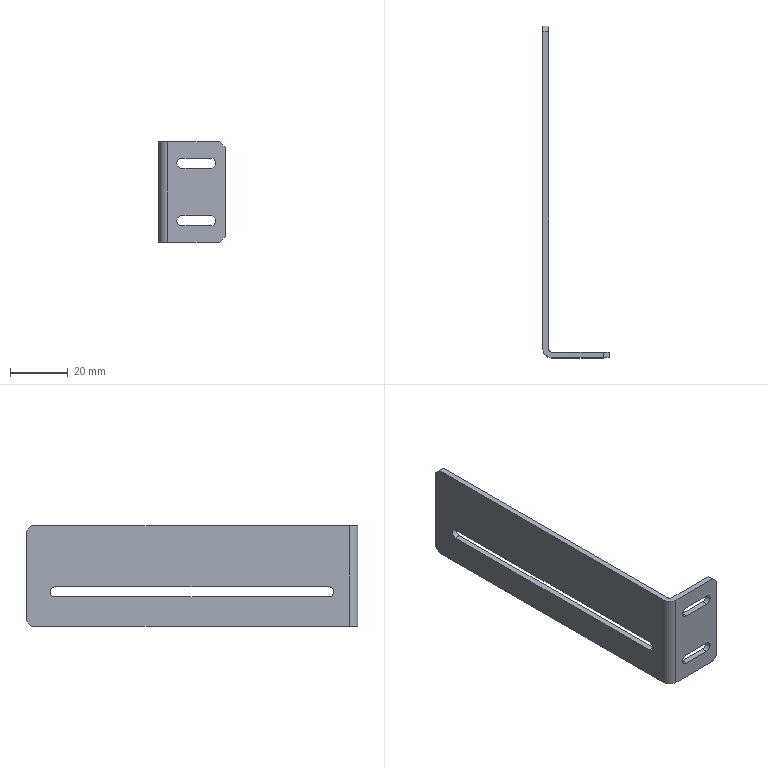Part | SolidWorks | features BaseBody 1 | 1 solid | 27 faces | box 23 x 115 x 35 mm | volume 8601 mm3 | plane 18 | cylinder 9 | commonest cylinder face diameters 3.5 x4 3.4 x3 2 x1 6 x1
STEP:
#1=CARTESIAN_POINT('',(-11.,6.3,-5.5));
#2=VERTEX_POINT('',#1);
#3=CARTESIAN_POINT('',(-11.,8.,-3.8));
#4=VERTEX_POINT('',#3);
#5=CARTESIAN_POINT('',(-11.,8.,-5.5));
#6=DIRECTION('',(-1.,0.,0.));
#7=DIRECTION('',(0.,1.,0.));
#8=AXIS2_PLACEMENT_3D('',#5,#6,#7);
#9=CIRCLE('',#8,1.7);
#10=EDGE_CURVE('',#2,#4,#9,.T.);
#11=ORIENTED_EDGE('',*,*,#10,.F.);
#12=CARTESIAN_POINT('',(-13.,6.3,-5.5));
#13=VERTEX_POINT('',#12);
#14=CARTESIAN_POINT('',(10.001,6.3,-5.5));
#15=DIRECTION('',(-1.,0.,0.));
#16=VECTOR('',#15,1000.);
#17=LINE('',#14,#16);
#18=EDGE_CURVE('',#2,#13,#17,.T.);
#19=ORIENTED_EDGE('',*,*,#18,.T.);
#20=CARTESIAN_POINT('',(-13.,8.,-3.8));
#21=VERTEX_POINT('',#20);
#22=CARTESIAN_POINT('',(-13.,8.,-5.5));
#23=DIRECTION('',(-1.,0.,0.));
#24=DIRECTION('',(0.,-1.,0.));
#25=AXIS2_PLACEMENT_3D('',#22,#23,#24);
#26=CIRCLE('',#25,1.7);
#27=EDGE_CURVE('',#13,#21,#26,.T.);
#28=ORIENTED_EDGE('',*,*,#27,.T.);
#29=CARTESIAN_POINT('',(10.001,8.,-3.8));
#30=DIRECTION('',(-1.,0.,0.));
#31=VECTOR('',#30,1000.);
#32=LINE('',#29,#31);
#33=EDGE_CURVE('',#4,#21,#32,.T.);
#34=ORIENTED_EDGE('',*,*,#33,.F.);
#35=EDGE_LOOP('',(#11,#19,#28,#34));
#36=FACE_OUTER_BOUND('',#35,.T.);
#37=CARTESIAN_POINT('',(10.001,8.,-5.5));
#38=DIRECTION('',(-1.,0.,0.));
#39=DIRECTION('',(0.,-1.,0.));
#40=AXIS2_PLACEMENT_3D('',#37,#38,#39);
#41=CYLINDRICAL_SURFACE('',#40,1.7);
#42=ADVANCED_FACE('',(#36),#41,.F.);
#43=ORIENTED_EDGE('',*,*,#33,.T.);
#44=CARTESIAN_POINT('',(-13.,103.,-3.8));
#45=VERTEX_POINT('',#44);
#46=CARTESIAN_POINT('',(-13.,8.,-3.8));
#47=DIRECTION('',(0.,1.,0.));
#48=VECTOR('',#47,1000.);
#49=LINE('',#46,#48);
#50=EDGE_CURVE('',#21,#45,#49,.T.);
#51=ORIENTED_EDGE('',*,*,#50,.T.);
#52=CARTESIAN_POINT('',(-11.,103.,-3.8));
#53=VERTEX_POINT('',#52);
#54=CARTESIAN_POINT('',(10.001,103.,-3.8));
#55=DIRECTION('',(-1.,0.,0.));
#56=VECTOR('',#55,1000.);
#57=LINE('',#54,#56);
#58=EDGE_CURVE('',#53,#45,#57,.T.);
#59=ORIENTED_EDGE('',*,*,#58,.F.);
#60=CARTESIAN_POINT('',(-11.,8.,-3.8));
#61=DIRECTION('',(0.,1.,0.));
#62=VECTOR('',#61,1000.);
#63=LINE('',#60,#62);
#64=EDGE_CURVE('',#4,#53,#63,.T.);
#65=ORIENTED_EDGE('',*,*,#64,.F.);
#66=EDGE_LOOP('',(#43,#51,#59,#65));
#67=FACE_OUTER_BOUND('',#66,.T.);
#68=CARTESIAN_POINT('',(10.001,8.,-3.8));
#69=DIRECTION('',(0.,0.,1.));
#70=DIRECTION('',(1.,0.,0.));
#71=AXIS2_PLACEMENT_3D('',#68,#69,#70);
#72=PLANE('',#71);
#73=ADVANCED_FACE('',(#67),#72,.F.);
#74=ORIENTED_EDGE('',*,*,#58,.T.);
#75=CARTESIAN_POINT('',(-13.,103.,-7.2));
#76=VERTEX_POINT('',#75);
#77=CARTESIAN_POINT('',(-13.,103.,-5.5));
#78=DIRECTION('',(-1.,0.,0.));
#79=DIRECTION('',(0.,-1.,0.));
#80=AXIS2_PLACEMENT_3D('',#77,#78,#79);
#81=CIRCLE('',#80,1.7);
#82=EDGE_CURVE('',#45,#76,#81,.T.);
#83=ORIENTED_EDGE('',*,*,#82,.T.);
#84=CARTESIAN_POINT('',(-11.,103.,-7.2));
#85=VERTEX_POINT('',#84);
#86=CARTESIAN_POINT('',(10.001,103.,-7.2));
#87=DIRECTION('',(-1.,0.,0.));
#88=VECTOR('',#87,1000.);
#89=LINE('',#86,#88);
#90=EDGE_CURVE('',#85,#76,#89,.T.);
#91=ORIENTED_EDGE('',*,*,#90,.F.);
#92=CARTESIAN_POINT('',(-11.,103.,-5.5));
#93=DIRECTION('',(-1.,0.,0.));
#94=DIRECTION('',(0.,1.,0.));
#95=AXIS2_PLACEMENT_3D('',#92,#93,#94);
#96=CIRCLE('',#95,1.7);
#97=EDGE_CURVE('',#53,#85,#96,.T.);
#98=ORIENTED_EDGE('',*,*,#97,.F.);
#99=EDGE_LOOP('',(#74,#83,#91,#98));
#100=FACE_OUTER_BOUND('',#99,.T.);
#101=CARTESIAN_POINT('',(10.001,103.,-5.5));
#102=DIRECTION('',(-1.,0.,0.));
#103=DIRECTION('',(0.,-1.,0.));
#104=AXIS2_PLACEMENT_3D('',#101,#102,#103);
#105=CYLINDRICAL_SURFACE('',#104,1.7);
#106=ADVANCED_FACE('',(#100),#105,.F.);
#107=ORIENTED_EDGE('',*,*,#90,.T.);
#108=CARTESIAN_POINT('',(-13.,8.,-7.2));
#109=VERTEX_POINT('',#108);
#110=CARTESIAN_POINT('',(-13.,8.,-7.2));
#111=DIRECTION('',(0.,-1.,0.));
#112=VECTOR('',#111,1000.);
#113=LINE('',#110,#112);
#114=EDGE_CURVE('',#76,#109,#113,.T.);
#115=ORIENTED_EDGE('',*,*,#114,.T.);
#116=CARTESIAN_POINT('',(-11.,8.,-7.2));
#117=VERTEX_POINT('',#116);
#118=CARTESIAN_POINT('',(10.001,8.,-7.2));
#119=DIRECTION('',(-1.,0.,0.));
#120=VECTOR('',#119,1000.);
#121=LINE('',#118,#120);
#122=EDGE_CURVE('',#117,#109,#121,.T.);
#123=ORIENTED_EDGE('',*,*,#122,.F.);
#124=CARTESIAN_POINT('',(-11.,8.,-7.2));
#125=DIRECTION('',(0.,-1.,0.));
#126=VECTOR('',#125,1000.);
#127=LINE('',#124,#126);
#128=EDGE_CURVE('',#85,#117,#127,.T.);
#129=ORIENTED_EDGE('',*,*,#128,.F.);
#130=EDGE_LOOP('',(#107,#115,#123,#129));
#131=FACE_OUTER_BOUND('',#130,.T.);
#132=CARTESIAN_POINT('',(10.001,8.,-7.2));
#133=DIRECTION('',(0.,0.,-1.));
#134=DIRECTION('',(-1.,0.,0.));
#135=AXIS2_PLACEMENT_3D('',#132,#133,#134);
#136=PLANE('',#135);
#137=ADVANCED_FACE('',(#131),#136,.F.);
#138=CARTESIAN_POINT('',(-13.,111.,17.5));
#139=VERTEX_POINT('',#138);
#140=CARTESIAN_POINT('',(-13.,113.,15.5));
#141=VERTEX_POINT('',#140);
#142=CARTESIAN_POINT('',(-13.,113.,15.5));
#143=DIRECTION('',(0.,0.7071,-0.7071));
#144=VECTOR('',#143,1000.);
#145=LINE('',#142,#144);
#146=EDGE_CURVE('',#139,#141,#145,.T.);
#147=ORIENTED_EDGE('',*,*,#146,.F.);
#148=CARTESIAN_POINT('',(-11.,111.,17.5));
#149=VERTEX_POINT('',#148);
#150=CARTESIAN_POINT('',(-13.,111.,17.5));
#151=DIRECTION('',(-1.,0.,0.));
#152=VECTOR('',#151,1000.);
#153=LINE('',#150,#152);
#154=EDGE_CURVE('',#149,#139,#153,.T.);
#155=ORIENTED_EDGE('',*,*,#154,.F.);
#156=CARTESIAN_POINT('',(-11.,113.,15.5));
#157=VERTEX_POINT('',#156);
#158=CARTESIAN_POINT('',(-11.,64.25,64.25));
#159=DIRECTION('',(0.,-0.7071,0.7071));
#160=VECTOR('',#159,1000.);
#161=LINE('',#158,#160);
#162=EDGE_CURVE('',#157,#149,#161,.T.);
#163=ORIENTED_EDGE('',*,*,#162,.F.);
#164=CARTESIAN_POINT('',(-13.,113.,15.5));
#165=DIRECTION('',(1.,0.,0.));
#166=VECTOR('',#165,1000.);
#167=LINE('',#164,#166);
#168=EDGE_CURVE('',#141,#157,#167,.T.);
#169=ORIENTED_EDGE('',*,*,#168,.F.);
#170=EDGE_LOOP('',(#147,#155,#163,#169));
#171=FACE_OUTER_BOUND('',#170,.T.);
#172=CARTESIAN_POINT('',(-13.,113.,15.5));
#173=DIRECTION('',(0.,-0.7071,-0.7071));
#174=DIRECTION('',(0.,-0.7071,0.7071));
#175=AXIS2_PLACEMENT_3D('',#172,#173,#174);
#176=PLANE('',#175);
#177=ADVANCED_FACE('',(#171),#176,.F.);
#178=CARTESIAN_POINT('',(-13.,113.,-15.5));
#179=VERTEX_POINT('',#178);
#180=CARTESIAN_POINT('',(-13.,111.,-17.5));
#181=VERTEX_POINT('',#180);
#182=CARTESIAN_POINT('',(-13.,111.,-17.5));
#183=DIRECTION('',(0.,-0.7071,-0.7071));
#184=VECTOR('',#183,1000.);
#185=LINE('',#182,#184);
#186=EDGE_CURVE('',#179,#181,#185,.T.);
#187=ORIENTED_EDGE('',*,*,#186,.F.);
#188=CARTESIAN_POINT('',(-11.,113.,-15.5));
#189=VERTEX_POINT('',#188);
#190=CARTESIAN_POINT('',(-13.,113.,-15.5));
#191=DIRECTION('',(-1.,0.,0.));
#192=VECTOR('',#191,1000.);
#193=LINE('',#190,#192);
#194=EDGE_CURVE('',#189,#179,#193,.T.);
#195=ORIENTED_EDGE('',*,*,#194,.F.);
#196=CARTESIAN_POINT('',(-11.,111.,-17.5));
#197=VERTEX_POINT('',#196);
#198=CARTESIAN_POINT('',(-11.,64.25,-64.25));
#199=DIRECTION('',(0.,0.7071,0.7071));
#200=VECTOR('',#199,1000.);
#201=LINE('',#198,#200);
#202=EDGE_CURVE('',#197,#189,#201,.T.);
#203=ORIENTED_EDGE('',*,*,#202,.F.);
#204=CARTESIAN_POINT('',(-13.,111.,-17.5));
#205=DIRECTION('',(1.,0.,0.));
#206=VECTOR('',#205,1000.);
#207=LINE('',#204,#206);
#208=EDGE_CURVE('',#181,#197,#207,.T.);
#209=ORIENTED_EDGE('',*,*,#208,.F.);
#210=EDGE_LOOP('',(#187,#195,#203,#209));
#211=FACE_OUTER_BOUND('',#210,.T.);
#212=CARTESIAN_POINT('',(-13.,111.,-17.5));
#213=DIRECTION('',(0.,-0.7071,0.7071));
#214=DIRECTION('',(-1.,0.,0.));
#215=AXIS2_PLACEMENT_3D('',#212,#213,#214);
#216=PLANE('',#215);
#217=ADVANCED_FACE('',(#211),#216,.F.);
#218=CARTESIAN_POINT('',(8.,-2.,-17.5));
#219=VERTEX_POINT('',#218);
#220=CARTESIAN_POINT('',(10.,-2.,-15.5));
#221=VERTEX_POINT('',#220);
#222=CARTESIAN_POINT('',(10.,-2.,-15.5));
#223=DIRECTION('',(0.7071,0.,0.7071));
#224=VECTOR('',#223,1000.);
#225=LINE('',#222,#224);
#226=EDGE_CURVE('',#219,#221,#225,.T.);
#227=ORIENTED_EDGE('',*,*,#226,.F.);
#228=CARTESIAN_POINT('',(8.,0.,-17.5));
#229=VERTEX_POINT('',#228);
#230=CARTESIAN_POINT('',(8.,-2.,-17.5));
#231=DIRECTION('',(0.,-1.,0.));
#232=VECTOR('',#231,1000.);
#233=LINE('',#230,#232);
#234=EDGE_CURVE('',#229,#219,#233,.T.);
#235=ORIENTED_EDGE('',*,*,#234,.F.);
#236=CARTESIAN_POINT('',(10.,0.,-15.5));
#237=VERTEX_POINT('',#236);
#238=CARTESIAN_POINT('',(12.75,0.,-12.75));
#239=DIRECTION('',(-0.7071,0.,-0.7071));
#240=VECTOR('',#239,1000.);
#241=LINE('',#238,#240);
#242=EDGE_CURVE('',#237,#229,#241,.T.);
#243=ORIENTED_EDGE('',*,*,#242,.F.);
#244=CARTESIAN_POINT('',(10.,-2.,-15.5));
#245=DIRECTION('',(0.,1.,0.));
#246=VECTOR('',#245,1000.);
#247=LINE('',#244,#246);
#248=EDGE_CURVE('',#221,#237,#247,.T.);
#249=ORIENTED_EDGE('',*,*,#248,.F.);
#250=EDGE_LOOP('',(#227,#235,#243,#249));
#251=FACE_OUTER_BOUND('',#250,.T.);
#252=CARTESIAN_POINT('',(10.,-2.,-15.5));
#253=DIRECTION('',(-0.7071,0.,0.7071));
#254=DIRECTION('',(0.,1.,0.));
#255=AXIS2_PLACEMENT_3D('',#252,#253,#254);
#256=PLANE('',#255);
#257=ADVANCED_FACE('',(#251),#256,.F.);
#258=CARTESIAN_POINT('',(10.,-2.,15.5));
#259=VERTEX_POINT('',#258);
#260=CARTESIAN_POINT('',(8.,-2.,17.5));
#261=VERTEX_POINT('',#260);
#262=CARTESIAN_POINT('',(8.,-2.,17.5));
#263=DIRECTION('',(-0.7071,0.,0.7071));
#264=VECTOR('',#263,1000.);
#265=LINE('',#262,#264);
#266=EDGE_CURVE('',#259,#261,#265,.T.);
#267=ORIENTED_EDGE('',*,*,#266,.F.);
#268=CARTESIAN_POINT('',(10.,0.,15.5));
#269=VERTEX_POINT('',#268);
#270=CARTESIAN_POINT('',(10.,-2.,15.5));
#271=DIRECTION('',(0.,-1.,0.));
#272=VECTOR('',#271,1000.);
#273=LINE('',#270,#272);
#274=EDGE_CURVE('',#269,#259,#273,.T.);
#275=ORIENTED_EDGE('',*,*,#274,.F.);
#276=CARTESIAN_POINT('',(8.,0.,17.5));
#277=VERTEX_POINT('',#276);
#278=CARTESIAN_POINT('',(12.75,0.,12.75));
#279=DIRECTION('',(0.7071,0.,-0.7071));
#280=VECTOR('',#279,1000.);
#281=LINE('',#278,#280);
#282=EDGE_CURVE('',#277,#269,#281,.T.);
#283=ORIENTED_EDGE('',*,*,#282,.F.);
#284=CARTESIAN_POINT('',(8.,-2.,17.5));
#285=DIRECTION('',(0.,1.,0.));
#286=VECTOR('',#285,1000.);
#287=LINE('',#284,#286);
#288=EDGE_CURVE('',#261,#277,#287,.T.);
#289=ORIENTED_EDGE('',*,*,#288,.F.);
#290=EDGE_LOOP('',(#267,#275,#283,#289));
#291=FACE_OUTER_BOUND('',#290,.T.);
#292=CARTESIAN_POINT('',(8.,-2.,17.5));
#293=DIRECTION('',(-0.7071,0.,-0.7071));
#294=DIRECTION('',(-0.7071,0.,0.7071));
#295=AXIS2_PLACEMENT_3D('',#292,#293,#294);
#296=PLANE('',#295);
#297=ADVANCED_FACE('',(#291),#296,.F.);
#298=CARTESIAN_POINT('',(5.,0.,11.75));
#299=VERTEX_POINT('',#298);
#300=CARTESIAN_POINT('',(5.,0.,8.25));
#301=VERTEX_POINT('',#300);
#302=CARTESIAN_POINT('',(5.,0.,10.));
#303=DIRECTION('',(0.,1.,0.));
#304=DIRECTION('',(0.,0.,1.));
#305=AXIS2_PLACEMENT_3D('',#302,#303,#304);
#306=CIRCLE('',#305,1.75);
#307=EDGE_CURVE('',#299,#301,#306,.T.);
#308=ORIENTED_EDGE('',*,*,#307,.T.);
#309=CARTESIAN_POINT('',(5.,-2.,8.25));
#310=VERTEX_POINT('',#309);
#311=CARTESIAN_POINT('',(5.,8.,8.25));
#312=DIRECTION('',(0.,-1.,0.));
#313=VECTOR('',#312,1000.);
#314=LINE('',#311,#313);
#315=EDGE_CURVE('',#301,#310,#314,.T.);
#316=ORIENTED_EDGE('',*,*,#315,.T.);
#317=CARTESIAN_POINT('',(5.,-2.,11.75));
#318=VERTEX_POINT('',#317);
#319=CARTESIAN_POINT('',(5.,-2.,10.));
#320=DIRECTION('',(0.,-1.,0.));
#321=DIRECTION('',(0.,0.,-1.));
#322=AXIS2_PLACEMENT_3D('',#319,#320,#321);
#323=CIRCLE('',#322,1.75);
#324=EDGE_CURVE('',#310,#318,#323,.T.);
#325=ORIENTED_EDGE('',*,*,#324,.T.);
#326=CARTESIAN_POINT('',(5.,8.,11.75));
#327=DIRECTION('',(0.,-1.,0.));
#328=VECTOR('',#327,1000.);
#329=LINE('',#326,#328);
#330=EDGE_CURVE('',#299,#318,#329,.T.);
#331=ORIENTED_EDGE('',*,*,#330,.F.);
#332=EDGE_LOOP('',(#308,#316,#325,#331));
#333=FACE_OUTER_BOUND('',#332,.T.);
#334=CARTESIAN_POINT('',(5.,8.,10.));
#335=DIRECTION('',(0.,-1.,0.));
#336=DIRECTION('',(0.,0.,-1.));
#337=AXIS2_PLACEMENT_3D('',#334,#335,#336);
#338=CYLINDRICAL_SURFACE('',#337,1.75);
#339=ADVANCED_FACE('',(#333),#338,.F.);
#340=CARTESIAN_POINT('',(-5.,0.,8.25));
#341=VERTEX_POINT('',#340);
#342=CARTESIAN_POINT('',(-5.,0.,11.75));
#343=VERTEX_POINT('',#342);
#344=CARTESIAN_POINT('',(-5.,0.,10.));
#345=DIRECTION('',(0.,1.,0.));
#346=DIRECTION('',(0.,0.,1.));
#347=AXIS2_PLACEMENT_3D('',#344,#345,#346);
#348=CIRCLE('',#347,1.75);
#349=EDGE_CURVE('',#341,#343,#348,.T.);
#350=ORIENTED_EDGE('',*,*,#349,.T.);
#351=CARTESIAN_POINT('',(-5.,-2.,11.75));
#352=VERTEX_POINT('',#351);
#353=CARTESIAN_POINT('',(-5.,8.,11.75));
#354=DIRECTION('',(0.,-1.,0.));
#355=VECTOR('',#354,1000.);
#356=LINE('',#353,#355);
#357=EDGE_CURVE('',#343,#352,#356,.T.);
#358=ORIENTED_EDGE('',*,*,#357,.T.);
#359=CARTESIAN_POINT('',(-5.,-2.,8.25));
#360=VERTEX_POINT('',#359);
#361=CARTESIAN_POINT('',(-5.,-2.,10.));
#362=DIRECTION('',(0.,-1.,0.));
#363=DIRECTION('',(0.,0.,-1.));
#364=AXIS2_PLACEMENT_3D('',#361,#362,#363);
#365=CIRCLE('',#364,1.75);
#366=EDGE_CURVE('',#352,#360,#365,.T.);
#367=ORIENTED_EDGE('',*,*,#366,.T.);
#368=CARTESIAN_POINT('',(-5.,8.,8.25));
#369=DIRECTION('',(0.,-1.,0.));
#370=VECTOR('',#369,1000.);
#371=LINE('',#368,#370);
#372=EDGE_CURVE('',#341,#360,#371,.T.);
#373=ORIENTED_EDGE('',*,*,#372,.F.);
#374=EDGE_LOOP('',(#350,#358,#367,#373));
#375=FACE_OUTER_BOUND('',#374,.T.);
#376=CARTESIAN_POINT('',(-5.,8.,10.));
#377=DIRECTION('',(0.,-1.,0.));
#378=DIRECTION('',(0.,0.,-1.));
#379=AXIS2_PLACEMENT_3D('',#376,#377,#378);
#380=CYLINDRICAL_SURFACE('',#379,1.75);
#381=ADVANCED_FACE('',(#375),#380,.F.);
#382=CARTESIAN_POINT('',(0.,0.,8.25));
#383=DIRECTION('',(-1.,0.,0.));
#384=VECTOR('',#383,1000.);
#385=LINE('',#382,#384);
#386=EDGE_CURVE('',#301,#341,#385,.T.);
#387=ORIENTED_EDGE('',*,*,#386,.T.);
#388=ORIENTED_EDGE('',*,*,#372,.T.);
#389=CARTESIAN_POINT('',(-5.,-2.,8.25));
#390=DIRECTION('',(1.,0.,0.));
#391=VECTOR('',#390,1000.);
#392=LINE('',#389,#391);
#393=EDGE_CURVE('',#360,#310,#392,.T.);
#394=ORIENTED_EDGE('',*,*,#393,.T.);
#395=ORIENTED_EDGE('',*,*,#315,.F.);
#396=EDGE_LOOP('',(#387,#388,#394,#395));
#397=FACE_OUTER_BOUND('',#396,.T.);
#398=CARTESIAN_POINT('',(-5.,8.,8.25));
#399=DIRECTION('',(0.,0.,-1.));
#400=DIRECTION('',(0.,-1.,0.));
#401=AXIS2_PLACEMENT_3D('',#398,#399,#400);
#402=PLANE('',#401);
#403=ADVANCED_FACE('',(#397),#402,.F.);
#404=CARTESIAN_POINT('',(0.,0.,11.75));
#405=DIRECTION('',(1.,0.,0.));
#406=VECTOR('',#405,1000.);
#407=LINE('',#404,#406);
#408=EDGE_CURVE('',#343,#299,#407,.T.);
#409=ORIENTED_EDGE('',*,*,#408,.T.);
#410=ORIENTED_EDGE('',*,*,#330,.T.);
#411=CARTESIAN_POINT('',(-5.,-2.,11.75));
#412=DIRECTION('',(-1.,0.,0.));
#413=VECTOR('',#412,1000.);
#414=LINE('',#411,#413);
#415=EDGE_CURVE('',#318,#352,#414,.T.);
#416=ORIENTED_EDGE('',*,*,#415,.T.);
#417=ORIENTED_EDGE('',*,*,#357,.F.);
#418=EDGE_LOOP('',(#409,#410,#416,#417));
#419=FACE_OUTER_BOUND('',#418,.T.);
#420=CARTESIAN_POINT('',(-5.,8.,11.75));
#421=DIRECTION('',(0.,0.,1.));
#422=DIRECTION('',(1.,0.,0.));
#423=AXIS2_PLACEMENT_3D('',#420,#421,#422);
#424=PLANE('',#423);
#425=ADVANCED_FACE('',(#419),#424,.F.);
#426=CARTESIAN_POINT('',(5.,0.,-8.25));
#427=VERTEX_POINT('',#426);
#428=CARTESIAN_POINT('',(5.,0.,-11.75));
#429=VERTEX_POINT('',#428);
#430=CARTESIAN_POINT('',(5.,0.,-10.));
#431=DIRECTION('',(0.,1.,0.));
#432=DIRECTION('',(0.,0.,1.));
#433=AXIS2_PLACEMENT_3D('',#430,#431,#432);
#434=CIRCLE('',#433,1.75);
#435=EDGE_CURVE('',#427,#429,#434,.T.);
#436=ORIENTED_EDGE('',*,*,#435,.T.);
#437=CARTESIAN_POINT('',(5.,-2.,-11.75));
#438=VERTEX_POINT('',#437);
#439=CARTESIAN_POINT('',(5.,8.,-11.75));
#440=DIRECTION('',(0.,-1.,0.));
#441=VECTOR('',#440,1000.);
#442=LINE('',#439,#441);
#443=EDGE_CURVE('',#429,#438,#442,.T.);
#444=ORIENTED_EDGE('',*,*,#443,.T.);
#445=CARTESIAN_POINT('',(5.,-2.,-8.25));
#446=VERTEX_POINT('',#445);
#447=CARTESIAN_POINT('',(5.,-2.,-10.));
#448=DIRECTION('',(0.,-1.,0.));
#449=DIRECTION('',(0.,0.,-1.));
#450=AXIS2_PLACEMENT_3D('',#447,#448,#449);
#451=CIRCLE('',#450,1.75);
#452=EDGE_CURVE('',#438,#446,#451,.T.);
#453=ORIENTED_EDGE('',*,*,#452,.T.);
#454=CARTESIAN_POINT('',(5.,8.,-8.25));
#455=DIRECTION('',(0.,-1.,0.));
#456=VECTOR('',#455,1000.);
#457=LINE('',#454,#456);
#458=EDGE_CURVE('',#427,#446,#457,.T.);
#459=ORIENTED_EDGE('',*,*,#458,.F.);
#460=EDGE_LOOP('',(#436,#444,#453,#459));
#461=FACE_OUTER_BOUND('',#460,.T.);
#462=CARTESIAN_POINT('',(5.,8.,-10.));
#463=DIRECTION('',(0.,-1.,0.));
#464=DIRECTION('',(0.,0.,-1.));
#465=AXIS2_PLACEMENT_3D('',#462,#463,#464);
#466=CYLINDRICAL_SURFACE('',#465,1.75);
#467=ADVANCED_FACE('',(#461),#466,.F.);
#468=CARTESIAN_POINT('',(-5.,0.,-11.75));
#469=VERTEX_POINT('',#468);
#470=CARTESIAN_POINT('',(-5.,0.,-8.25));
#471=VERTEX_POINT('',#470);
#472=CARTESIAN_POINT('',(-5.,0.,-10.));
#473=DIRECTION('',(0.,1.,0.));
#474=DIRECTION('',(0.,0.,1.));
#475=AXIS2_PLACEMENT_3D('',#472,#473,#474);
#476=CIRCLE('',#475,1.75);
#477=EDGE_CURVE('',#469,#471,#476,.T.);
#478=ORIENTED_EDGE('',*,*,#477,.T.);
#479=CARTESIAN_POINT('',(-5.,-2.,-8.25));
#480=VERTEX_POINT('',#479);
#481=CARTESIAN_POINT('',(-5.,8.,-8.25));
#482=DIRECTION('',(0.,-1.,0.));
#483=VECTOR('',#482,1000.);
#484=LINE('',#481,#483);
#485=EDGE_CURVE('',#471,#480,#484,.T.);
#486=ORIENTED_EDGE('',*,*,#485,.T.);
#487=CARTESIAN_POINT('',(-5.,-2.,-11.75));
#488=VERTEX_POINT('',#487);
#489=CARTESIAN_POINT('',(-5.,-2.,-10.));
#490=DIRECTION('',(0.,-1.,0.));
#491=DIRECTION('',(0.,0.,-1.));
#492=AXIS2_PLACEMENT_3D('',#489,#490,#491);
#493=CIRCLE('',#492,1.75);
#494=EDGE_CURVE('',#480,#488,#493,.T.);
#495=ORIENTED_EDGE('',*,*,#494,.T.);
#496=CARTESIAN_POINT('',(-5.,8.,-11.75));
#497=DIRECTION('',(0.,-1.,0.));
#498=VECTOR('',#497,1000.);
#499=LINE('',#496,#498);
#500=EDGE_CURVE('',#469,#488,#499,.T.);
#501=ORIENTED_EDGE('',*,*,#500,.F.);
#502=EDGE_LOOP('',(#478,#486,#495,#501));
#503=FACE_OUTER_BOUND('',#502,.T.);
#504=CARTESIAN_POINT('',(-5.,8.,-10.));
#505=DIRECTION('',(0.,-1.,0.));
#506=DIRECTION('',(0.,0.,-1.));
#507=AXIS2_PLACEMENT_3D('',#504,#505,#506);
#508=CYLINDRICAL_SURFACE('',#507,1.75);
#509=ADVANCED_FACE('',(#503),#508,.F.);
#510=CARTESIAN_POINT('',(0.,0.,-11.75));
#511=DIRECTION('',(-1.,0.,0.));
#512=VECTOR('',#511,1000.);
#513=LINE('',#510,#512);
#514=EDGE_CURVE('',#429,#469,#513,.T.);
#515=ORIENTED_EDGE('',*,*,#514,.T.);
#516=ORIENTED_EDGE('',*,*,#500,.T.);
#517=CARTESIAN_POINT('',(-5.,-2.,-11.75));
#518=DIRECTION('',(1.,0.,0.));
#519=VECTOR('',#518,1000.);
#520=LINE('',#517,#519);
#521=EDGE_CURVE('',#488,#438,#520,.T.);
#522=ORIENTED_EDGE('',*,*,#521,.T.);
#523=ORIENTED_EDGE('',*,*,#443,.F.);
#524=EDGE_LOOP('',(#515,#516,#522,#523));
#525=FACE_OUTER_BOUND('',#524,.T.);
#526=CARTESIAN_POINT('',(-5.,8.,-11.75));
#527=DIRECTION('',(0.,0.,-1.));
#528=DIRECTION('',(0.,-1.,0.));
#529=AXIS2_PLACEMENT_3D('',#526,#527,#528);
#530=PLANE('',#529);
#531=ADVANCED_FACE('',(#525),#530,.F.);
#532=CARTESIAN_POINT('',(0.,0.,-8.25));
#533=DIRECTION('',(1.,0.,0.));
#534=VECTOR('',#533,1000.);
#535=LINE('',#532,#534);
#536=EDGE_CURVE('',#471,#427,#535,.T.);
#537=ORIENTED_EDGE('',*,*,#536,.T.);
#538=ORIENTED_EDGE('',*,*,#458,.T.);
#539=CARTESIAN_POINT('',(-5.,-2.,-8.25));
#540=DIRECTION('',(-1.,0.,0.));
#541=VECTOR('',#540,1000.);
#542=LINE('',#539,#541);
#543=EDGE_CURVE('',#446,#480,#542,.T.);
#544=ORIENTED_EDGE('',*,*,#543,.T.);
#545=ORIENTED_EDGE('',*,*,#485,.F.);
#546=EDGE_LOOP('',(#537,#538,#544,#545));
#547=FACE_OUTER_BOUND('',#546,.T.);
#548=CARTESIAN_POINT('',(-5.,8.,-8.25));
#549=DIRECTION('',(0.,0.,1.));
#550=DIRECTION('',(1.,0.,0.));
#551=AXIS2_PLACEMENT_3D('',#548,#549,#550);
#552=PLANE('',#551);
#553=ADVANCED_FACE('',(#547),#552,.F.);
#554=CARTESIAN_POINT('',(-11.,113.,-17.5));
#555=DIRECTION('',(0.,0.,-1.));
#556=VECTOR('',#555,1000.);
#557=LINE('',#554,#556);
#558=EDGE_CURVE('',#157,#189,#557,.T.);
#559=ORIENTED_EDGE('',*,*,#558,.T.);
#560=ORIENTED_EDGE('',*,*,#194,.T.);
#561=CARTESIAN_POINT('',(-13.,113.,0.));
#562=DIRECTION('',(0.,0.,-1.));
#563=VECTOR('',#562,1000.);
#564=LINE('',#561,#563);
#565=EDGE_CURVE('',#141,#179,#564,.T.);
#566=ORIENTED_EDGE('',*,*,#565,.F.);
#567=ORIENTED_EDGE('',*,*,#168,.T.);
#568=EDGE_LOOP('',(#559,#560,#566,#567));
#569=FACE_OUTER_BOUND('',#568,.T.);
#570=CARTESIAN_POINT('',(-13.,113.,-17.5));
#571=DIRECTION('',(0.,-1.,0.));
#572=DIRECTION('',(0.,0.,-1.));
#573=AXIS2_PLACEMENT_3D('',#570,#571,#572);
#574=PLANE('',#573);
#575=ADVANCED_FACE('',(#569),#574,.F.);
#576=ORIENTED_EDGE('',*,*,#128,.T.);
#577=CARTESIAN_POINT('',(-11.,8.,-5.5));
#578=DIRECTION('',(-1.,0.,0.));
#579=DIRECTION('',(0.,1.,0.));
#580=AXIS2_PLACEMENT_3D('',#577,#578,#579);
#581=CIRCLE('',#580,1.7);
#582=EDGE_CURVE('',#117,#2,#581,.T.);
#583=ORIENTED_EDGE('',*,*,#582,.T.);
#584=ORIENTED_EDGE('',*,*,#10,.T.);
#585=ORIENTED_EDGE('',*,*,#64,.T.);
#586=ORIENTED_EDGE('',*,*,#97,.T.);
#587=EDGE_LOOP('',(#576,#583,#584,#585,#586));
#588=FACE_BOUND('',#587,.T.);
#589=CARTESIAN_POINT('',(-11.,1.,-17.5));
#590=VERTEX_POINT('',#589);
#591=CARTESIAN_POINT('',(-11.,0.,-17.5));
#592=DIRECTION('',(0.,-1.,0.));
#593=VECTOR('',#592,1000.);
#594=LINE('',#591,#593);
#595=EDGE_CURVE('',#197,#590,#594,.T.);
#596=ORIENTED_EDGE('',*,*,#595,.F.);
#597=ORIENTED_EDGE('',*,*,#202,.T.);
#598=ORIENTED_EDGE('',*,*,#558,.F.);
#599=ORIENTED_EDGE('',*,*,#162,.T.);
#600=CARTESIAN_POINT('',(-11.,1.,17.5));
#601=VERTEX_POINT('',#600);
#602=CARTESIAN_POINT('',(-11.,113.,17.5));
#603=DIRECTION('',(0.,1.,0.));
#604=VECTOR('',#603,1000.);
#605=LINE('',#602,#604);
#606=EDGE_CURVE('',#601,#149,#605,.T.);
#607=ORIENTED_EDGE('',*,*,#606,.F.);
#608=CARTESIAN_POINT('',(-11.,1.,-17.5));
#609=DIRECTION('',(0.,0.,1.));
#610=VECTOR('',#609,1000.);
#611=LINE('',#608,#610);
#612=EDGE_CURVE('',#590,#601,#611,.T.);
#613=ORIENTED_EDGE('',*,*,#612,.F.);
#614=EDGE_LOOP('',(#596,#597,#598,#599,#607,#613));
#615=FACE_OUTER_BOUND('',#614,.T.);
#616=CARTESIAN_POINT('',(-11.,0.,0.));
#617=DIRECTION('',(1.,0.,0.));
#618=DIRECTION('',(0.,1.,0.));
#619=AXIS2_PLACEMENT_3D('',#616,#617,#618);
#620=PLANE('',#619);
#621=ADVANCED_FACE('',(#588,#615),#620,.T.);
#622=ORIENTED_EDGE('',*,*,#50,.F.);
#623=ORIENTED_EDGE('',*,*,#27,.F.);
#624=CARTESIAN_POINT('',(-13.,8.,-5.5));
#625=DIRECTION('',(-1.,0.,0.));
#626=DIRECTION('',(0.,-1.,0.));
#627=AXIS2_PLACEMENT_3D('',#624,#625,#626);
#628=CIRCLE('',#627,1.7);
#629=EDGE_CURVE('',#109,#13,#628,.T.);
#630=ORIENTED_EDGE('',*,*,#629,.F.);
#631=ORIENTED_EDGE('',*,*,#114,.F.);
#632=ORIENTED_EDGE('',*,*,#82,.F.);
#633=EDGE_LOOP('',(#622,#623,#630,#631,#632));
#634=FACE_BOUND('',#633,.T.);
#635=ORIENTED_EDGE('',*,*,#565,.T.);
#636=ORIENTED_EDGE('',*,*,#186,.T.);
#637=CARTESIAN_POINT('',(-13.,1.,-17.5));
#638=VERTEX_POINT('',#637);
#639=CARTESIAN_POINT('',(-13.,0.,-17.5));
#640=DIRECTION('',(0.,-1.,0.));
#641=VECTOR('',#640,1000.);
#642=LINE('',#639,#641);
#643=EDGE_CURVE('',#181,#638,#642,.T.);
#644=ORIENTED_EDGE('',*,*,#643,.T.);
#645=CARTESIAN_POINT('',(-13.,1.,17.5));
#646=VERTEX_POINT('',#645);
#647=CARTESIAN_POINT('',(-13.,1.,-17.5));
#648=DIRECTION('',(0.,0.,-1.));
#649=VECTOR('',#648,1000.);
#650=LINE('',#647,#649);
#651=EDGE_CURVE('',#646,#638,#650,.T.);
#652=ORIENTED_EDGE('',*,*,#651,.F.);
#653=CARTESIAN_POINT('',(-13.,0.,17.5));
#654=DIRECTION('',(0.,1.,0.));
#655=VECTOR('',#654,1000.);
#656=LINE('',#653,#655);
#657=EDGE_CURVE('',#646,#139,#656,.T.);
#658=ORIENTED_EDGE('',*,*,#657,.T.);
#659=ORIENTED_EDGE('',*,*,#146,.T.);
#660=EDGE_LOOP('',(#635,#636,#644,#652,#658,#659));
#661=FACE_OUTER_BOUND('',#660,.T.);
#662=CARTESIAN_POINT('',(-13.,0.,0.));
#663=DIRECTION('',(1.,0.,0.));
#664=DIRECTION('',(0.,1.,0.));
#665=AXIS2_PLACEMENT_3D('',#662,#663,#664);
#666=PLANE('',#665);
#667=ADVANCED_FACE('',(#634,#661),#666,.F.);
#668=CARTESIAN_POINT('',(-10.,0.,-17.5));
#669=VERTEX_POINT('',#668);
#670=CARTESIAN_POINT('',(-10.,0.,17.5));
#671=VERTEX_POINT('',#670);
#672=CARTESIAN_POINT('',(-10.,0.,-17.5));
#673=DIRECTION('',(0.,0.,1.));
#674=VECTOR('',#673,1000.);
#675=LINE('',#672,#674);
#676=EDGE_CURVE('',#669,#671,#675,.T.);
#677=ORIENTED_EDGE('',*,*,#676,.F.);
#678=CARTESIAN_POINT('',(-10.,1.,-17.5));
#679=DIRECTION('',(0.,0.,-1.));
#680=DIRECTION('',(1.,0.,0.));
#681=AXIS2_PLACEMENT_3D('',#678,#679,#680);
#682=CIRCLE('',#681,1.);
#683=EDGE_CURVE('',#669,#590,#682,.T.);
#684=ORIENTED_EDGE('',*,*,#683,.T.);
#685=ORIENTED_EDGE('',*,*,#612,.T.);
#686=CARTESIAN_POINT('',(-10.,1.,17.5));
#687=DIRECTION('',(0.,0.,1.));
#688=DIRECTION('',(1.,0.,0.));
#689=AXIS2_PLACEMENT_3D('',#686,#687,#688);
#690=CIRCLE('',#689,1.);
#691=EDGE_CURVE('',#601,#671,#690,.T.);
#692=ORIENTED_EDGE('',*,*,#691,.T.);
#693=EDGE_LOOP('',(#677,#684,#685,#692));
#694=FACE_OUTER_BOUND('',#693,.T.);
#695=CARTESIAN_POINT('',(-10.,1.,17.5));
#696=DIRECTION('',(0.,0.,1.));
#697=DIRECTION('',(-1.,0.,0.));
#698=AXIS2_PLACEMENT_3D('',#695,#696,#697);
#699=CYLINDRICAL_SURFACE('',#698,1.);
#700=ADVANCED_FACE('',(#694),#699,.F.);
#701=CARTESIAN_POINT('',(-10.,-2.,-17.5));
#702=VERTEX_POINT('',#701);
#703=CARTESIAN_POINT('',(-10.,-2.,17.5));
#704=VERTEX_POINT('',#703);
#705=CARTESIAN_POINT('',(-10.,-2.,-17.5));
#706=DIRECTION('',(0.,0.,1.));
#707=VECTOR('',#706,1000.);
#708=LINE('',#705,#707);
#709=EDGE_CURVE('',#702,#704,#708,.T.);
#710=ORIENTED_EDGE('',*,*,#709,.T.);
#711=CARTESIAN_POINT('',(-10.,1.,17.5));
#712=DIRECTION('',(0.,0.,1.));
#713=DIRECTION('',(1.,0.,0.));
#714=AXIS2_PLACEMENT_3D('',#711,#712,#713);
#715=CIRCLE('',#714,3.);
#716=EDGE_CURVE('',#646,#704,#715,.T.);
#717=ORIENTED_EDGE('',*,*,#716,.F.);
#718=ORIENTED_EDGE('',*,*,#651,.T.);
#719=CARTESIAN_POINT('',(-10.,1.,-17.5));
#720=DIRECTION('',(0.,0.,-1.));
#721=DIRECTION('',(1.,0.,0.));
#722=AXIS2_PLACEMENT_3D('',#719,#720,#721);
#723=CIRCLE('',#722,3.);
#724=EDGE_CURVE('',#702,#638,#723,.T.);
#725=ORIENTED_EDGE('',*,*,#724,.F.);
#726=EDGE_LOOP('',(#710,#717,#718,#725));
#727=FACE_OUTER_BOUND('',#726,.T.);
#728=CARTESIAN_POINT('',(-10.,1.,17.5));
#729=DIRECTION('',(0.,0.,1.));
#730=DIRECTION('',(-1.,0.,0.));
#731=AXIS2_PLACEMENT_3D('',#728,#729,#730);
#732=CYLINDRICAL_SURFACE('',#731,3.);
#733=ADVANCED_FACE('',(#727),#732,.T.);
#734=ORIENTED_EDGE('',*,*,#477,.F.);
#735=ORIENTED_EDGE('',*,*,#514,.F.);
#736=ORIENTED_EDGE('',*,*,#435,.F.);
#737=ORIENTED_EDGE('',*,*,#536,.F.);
#738=EDGE_LOOP('',(#734,#735,#736,#737));
#739=FACE_BOUND('',#738,.T.);
#740=ORIENTED_EDGE('',*,*,#349,.F.);
#741=ORIENTED_EDGE('',*,*,#386,.F.);
#742=ORIENTED_EDGE('',*,*,#307,.F.);
#743=ORIENTED_EDGE('',*,*,#408,.F.);
#744=EDGE_LOOP('',(#740,#741,#742,#743));
#745=FACE_BOUND('',#744,.T.);
#746=CARTESIAN_POINT('',(-10.,0.,17.5));
#747=DIRECTION('',(1.,0.,0.));
#748=VECTOR('',#747,1000.);
#749=LINE('',#746,#748);
#750=EDGE_CURVE('',#671,#277,#749,.T.);
#751=ORIENTED_EDGE('',*,*,#750,.T.);
#752=ORIENTED_EDGE('',*,*,#282,.T.);
#753=CARTESIAN_POINT('',(10.,0.,-17.5));
#754=DIRECTION('',(0.,0.,-1.));
#755=VECTOR('',#754,1000.);
#756=LINE('',#753,#755);
#757=EDGE_CURVE('',#269,#237,#756,.T.);
#758=ORIENTED_EDGE('',*,*,#757,.T.);
#759=ORIENTED_EDGE('',*,*,#242,.T.);
#760=CARTESIAN_POINT('',(-10.,0.,-17.5));
#761=DIRECTION('',(-1.,0.,0.));
#762=VECTOR('',#761,1000.);
#763=LINE('',#760,#762);
#764=EDGE_CURVE('',#229,#669,#763,.T.);
#765=ORIENTED_EDGE('',*,*,#764,.T.);
#766=ORIENTED_EDGE('',*,*,#676,.T.);
#767=EDGE_LOOP('',(#751,#752,#758,#759,#765,#766));
#768=FACE_OUTER_BOUND('',#767,.T.);
#769=CARTESIAN_POINT('',(0.,0.,0.));
#770=DIRECTION('',(0.,1.,0.));
#771=DIRECTION('',(1.,0.,0.));
#772=AXIS2_PLACEMENT_3D('',#769,#770,#771);
#773=PLANE('',#772);
#774=ADVANCED_FACE('',(#739,#745,#768),#773,.T.);
#775=ORIENTED_EDGE('',*,*,#393,.F.);
#776=ORIENTED_EDGE('',*,*,#366,.F.);
#777=ORIENTED_EDGE('',*,*,#415,.F.);
#778=ORIENTED_EDGE('',*,*,#324,.F.);
#779=EDGE_LOOP('',(#775,#776,#777,#778));
#780=FACE_BOUND('',#779,.T.);
#781=ORIENTED_EDGE('',*,*,#521,.F.);
#782=ORIENTED_EDGE('',*,*,#494,.F.);
#783=ORIENTED_EDGE('',*,*,#543,.F.);
#784=ORIENTED_EDGE('',*,*,#452,.F.);
#785=EDGE_LOOP('',(#781,#782,#783,#784));
#786=FACE_BOUND('',#785,.T.);
#787=CARTESIAN_POINT('',(10.,-2.,-17.5));
#788=DIRECTION('',(0.,0.,-1.));
#789=VECTOR('',#788,1000.);
#790=LINE('',#787,#789);
#791=EDGE_CURVE('',#259,#221,#790,.T.);
#792=ORIENTED_EDGE('',*,*,#791,.F.);
#793=ORIENTED_EDGE('',*,*,#266,.T.);
#794=CARTESIAN_POINT('',(-10.,-2.,17.5));
#795=DIRECTION('',(1.,0.,0.));
#796=VECTOR('',#795,1000.);
#797=LINE('',#794,#796);
#798=EDGE_CURVE('',#704,#261,#797,.T.);
#799=ORIENTED_EDGE('',*,*,#798,.F.);
#800=ORIENTED_EDGE('',*,*,#709,.F.);
#801=CARTESIAN_POINT('',(-10.,-2.,-17.5));
#802=DIRECTION('',(-1.,0.,0.));
#803=VECTOR('',#802,1000.);
#804=LINE('',#801,#803);
#805=EDGE_CURVE('',#219,#702,#804,.T.);
#806=ORIENTED_EDGE('',*,*,#805,.F.);
#807=ORIENTED_EDGE('',*,*,#226,.T.);
#808=EDGE_LOOP('',(#792,#793,#799,#800,#806,#807));
#809=FACE_OUTER_BOUND('',#808,.T.);
#810=CARTESIAN_POINT('',(0.,-2.,0.));
#811=DIRECTION('',(0.,1.,0.));
#812=DIRECTION('',(1.,0.,0.));
#813=AXIS2_PLACEMENT_3D('',#810,#811,#812);
#814=PLANE('',#813);
#815=ADVANCED_FACE('',(#780,#786,#809),#814,.F.);
#816=ORIENTED_EDGE('',*,*,#764,.F.);
#817=ORIENTED_EDGE('',*,*,#234,.T.);
#818=ORIENTED_EDGE('',*,*,#805,.T.);
#819=ORIENTED_EDGE('',*,*,#724,.T.);
#820=ORIENTED_EDGE('',*,*,#643,.F.);
#821=ORIENTED_EDGE('',*,*,#208,.T.);
#822=ORIENTED_EDGE('',*,*,#595,.T.);
#823=ORIENTED_EDGE('',*,*,#683,.F.);
#824=EDGE_LOOP('',(#816,#817,#818,#819,#820,#821,#822,#823));
#825=FACE_OUTER_BOUND('',#824,.T.);
#826=CARTESIAN_POINT('',(-10.,-2.,-17.5));
#827=DIRECTION('',(0.,0.,-1.));
#828=DIRECTION('',(0.,-1.,0.));
#829=AXIS2_PLACEMENT_3D('',#826,#827,#828);
#830=PLANE('',#829);
#831=ADVANCED_FACE('',(#825),#830,.T.);
#832=ORIENTED_EDGE('',*,*,#798,.T.);
#833=ORIENTED_EDGE('',*,*,#288,.T.);
#834=ORIENTED_EDGE('',*,*,#750,.F.);
#835=ORIENTED_EDGE('',*,*,#691,.F.);
#836=ORIENTED_EDGE('',*,*,#606,.T.);
#837=ORIENTED_EDGE('',*,*,#154,.T.);
#838=ORIENTED_EDGE('',*,*,#657,.F.);
#839=ORIENTED_EDGE('',*,*,#716,.T.);
#840=EDGE_LOOP('',(#832,#833,#834,#835,#836,#837,#838,#839));
#841=FACE_OUTER_BOUND('',#840,.T.);
#842=CARTESIAN_POINT('',(-10.,-2.,17.5));
#843=DIRECTION('',(0.,0.,1.));
#844=DIRECTION('',(1.,0.,0.));
#845=AXIS2_PLACEMENT_3D('',#842,#843,#844);
#846=PLANE('',#845);
#847=ADVANCED_FACE('',(#841),#846,.T.);
#848=ORIENTED_EDGE('',*,*,#757,.F.);
#849=ORIENTED_EDGE('',*,*,#274,.T.);
#850=ORIENTED_EDGE('',*,*,#791,.T.);
#851=ORIENTED_EDGE('',*,*,#248,.T.);
#852=EDGE_LOOP('',(#848,#849,#850,#851));
#853=FACE_OUTER_BOUND('',#852,.T.);
#854=CARTESIAN_POINT('',(10.,-2.,-17.5));
#855=DIRECTION('',(1.,0.,0.));
#856=DIRECTION('',(0.,0.,-1.));
#857=AXIS2_PLACEMENT_3D('',#854,#855,#856);
#858=PLANE('',#857);
#859=ADVANCED_FACE('',(#853),#858,.T.);
#860=ORIENTED_EDGE('',*,*,#18,.F.);
#861=ORIENTED_EDGE('',*,*,#582,.F.);
#862=ORIENTED_EDGE('',*,*,#122,.T.);
#863=ORIENTED_EDGE('',*,*,#629,.T.);
#864=EDGE_LOOP('',(#860,#861,#862,#863));
#865=FACE_OUTER_BOUND('',#864,.T.);
#866=CARTESIAN_POINT('',(10.001,8.,-5.5));
#867=DIRECTION('',(-1.,0.,0.));
#868=DIRECTION('',(0.,-1.,0.));
#869=AXIS2_PLACEMENT_3D('',#866,#867,#868);
#870=CYLINDRICAL_SURFACE('',#869,1.7);
#871=ADVANCED_FACE('',(#865),#870,.F.);
#872=CLOSED_SHELL('',(#42,#73,#106,#137,#177,#217,#257,#297,#339,#381,#403,#425,#467,#509,#531,#553,#575,#621,#667,#700,#733,#774,#815,#831,#847,#859,#871));
#873=MANIFOLD_SOLID_BREP('',#872);
#874=CARTESIAN_POINT('',(0.,0.,0.));
#875=DIRECTION('',(0.,0.,1.));
#876=DIRECTION('',(1.,0.,0.));
#877=AXIS2_PLACEMENT_3D('',#874,#875,#876);
#878=(LENGTH_UNIT()NAMED_UNIT(*)SI_UNIT(.MILLI.,.METRE.));
#879=UNCERTAINTY_MEASURE_WITH_UNIT(LENGTH_MEASURE(0.00001),#878,'','');
#880=(NAMED_UNIT(*)PLANE_ANGLE_UNIT()SI_UNIT($,.RADIAN.));
#881=(NAMED_UNIT(*)SI_UNIT($,.STERADIAN.)SOLID_ANGLE_UNIT());
#882=(GEOMETRIC_REPRESENTATION_CONTEXT(3)GLOBAL_UNCERTAINTY_ASSIGNED_CONTEXT((#879))GLOBAL_UNIT_ASSIGNED_CONTEXT((#878,#880,#881))REPRESENTATION_CONTEXT('',''));
#883=ADVANCED_BREP_SHAPE_REPRESENTATION('',(#873,#877),#882);